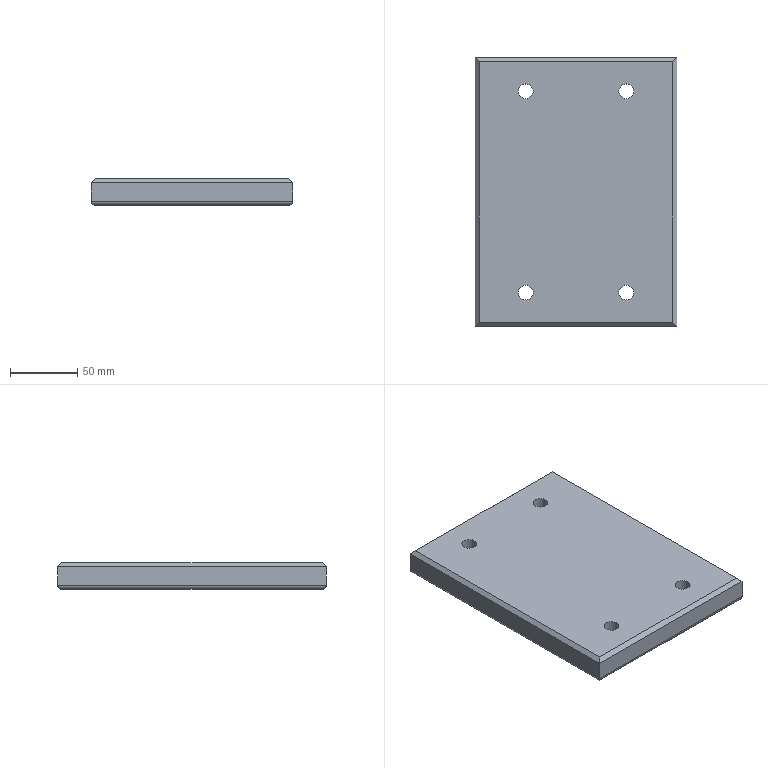Part | NX | features solid 2 | 1 solid | 26 faces | box 150 x 200 x 20 mm | volume 580958 mm3 | plane 14 | cylinder 12 | commonest cylinder face diameters 6 x4 11 x4 17.5 x4
STEP:
#1=CARTESIAN_POINT('',(660.,-340.,317.));
#2=VERTEX_POINT('',#1);
#3=CARTESIAN_POINT('',(660.,-340.,303.));
#4=VERTEX_POINT('',#3);
#5=CARTESIAN_POINT('',(660.,-340.,320.));
#6=DIRECTION('',(0.,0.,-1.));
#7=VECTOR('',#6,1000.);
#8=LINE('',#5,#7);
#9=EDGE_CURVE('',#2,#4,#8,.T.);
#10=ORIENTED_EDGE('',*,*,#9,.T.);
#11=CARTESIAN_POINT('',(510.,-340.,303.));
#12=VERTEX_POINT('',#11);
#13=CARTESIAN_POINT('',(660.,-340.,303.));
#14=DIRECTION('',(1.,0.,0.));
#15=VECTOR('',#14,1000.);
#16=LINE('',#13,#15);
#17=EDGE_CURVE('',#12,#4,#16,.T.);
#18=ORIENTED_EDGE('',*,*,#17,.F.);
#19=CARTESIAN_POINT('',(510.,-340.,317.));
#20=VERTEX_POINT('',#19);
#21=CARTESIAN_POINT('',(510.,-340.,320.));
#22=DIRECTION('',(0.,0.,-1.));
#23=VECTOR('',#22,1000.);
#24=LINE('',#21,#23);
#25=EDGE_CURVE('',#20,#12,#24,.T.);
#26=ORIENTED_EDGE('',*,*,#25,.F.);
#27=CARTESIAN_POINT('',(535.,-340.,317.));
#28=DIRECTION('',(-1.,0.,0.));
#29=VECTOR('',#28,1000.);
#30=LINE('',#27,#29);
#31=EDGE_CURVE('',#2,#20,#30,.T.);
#32=ORIENTED_EDGE('',*,*,#31,.F.);
#33=EDGE_LOOP('',(#10,#18,#26,#32));
#34=FACE_BOUND('',#33,.T.);
#35=CARTESIAN_POINT('',(535.,-340.,320.));
#36=DIRECTION('',(0.,-1.,0.));
#37=DIRECTION('',(-1.,0.,0.));
#38=AXIS2_PLACEMENT_3D('',#35,#36,#37);
#39=PLANE('',#38);
#40=ADVANCED_FACE('',(#34),#39,.F.);
#41=CARTESIAN_POINT('',(660.,-540.,317.));
#42=VERTEX_POINT('',#41);
#43=CARTESIAN_POINT('',(660.,-540.,303.));
#44=VERTEX_POINT('',#43);
#45=CARTESIAN_POINT('',(660.,-540.,320.));
#46=DIRECTION('',(0.,0.,-1.));
#47=VECTOR('',#46,1000.);
#48=LINE('',#45,#47);
#49=EDGE_CURVE('',#42,#44,#48,.T.);
#50=ORIENTED_EDGE('',*,*,#49,.T.);
#51=CARTESIAN_POINT('',(660.,-540.,303.));
#52=DIRECTION('',(0.,-1.,0.));
#53=VECTOR('',#52,1000.);
#54=LINE('',#51,#53);
#55=EDGE_CURVE('',#4,#44,#54,.T.);
#56=ORIENTED_EDGE('',*,*,#55,.F.);
#57=ORIENTED_EDGE('',*,*,#9,.F.);
#58=CARTESIAN_POINT('',(660.,-340.,317.));
#59=DIRECTION('',(0.,1.,0.));
#60=VECTOR('',#59,1000.);
#61=LINE('',#58,#60);
#62=EDGE_CURVE('',#42,#2,#61,.T.);
#63=ORIENTED_EDGE('',*,*,#62,.F.);
#64=EDGE_LOOP('',(#50,#56,#57,#63));
#65=FACE_BOUND('',#64,.T.);
#66=CARTESIAN_POINT('',(660.,-340.,320.));
#67=DIRECTION('',(-1.,0.,0.));
#68=DIRECTION('',(0.,0.,1.));
#69=AXIS2_PLACEMENT_3D('',#66,#67,#68);
#70=PLANE('',#69);
#71=ADVANCED_FACE('',(#65),#70,.F.);
#72=CARTESIAN_POINT('',(510.,-540.,317.));
#73=VERTEX_POINT('',#72);
#74=CARTESIAN_POINT('',(510.,-540.,303.));
#75=VERTEX_POINT('',#74);
#76=CARTESIAN_POINT('',(510.,-540.,320.));
#77=DIRECTION('',(0.,0.,-1.));
#78=VECTOR('',#77,1000.);
#79=LINE('',#76,#78);
#80=EDGE_CURVE('',#73,#75,#79,.T.);
#81=ORIENTED_EDGE('',*,*,#80,.T.);
#82=CARTESIAN_POINT('',(535.,-540.,303.));
#83=DIRECTION('',(-1.,0.,0.));
#84=VECTOR('',#83,1000.);
#85=LINE('',#82,#84);
#86=EDGE_CURVE('',#44,#75,#85,.T.);
#87=ORIENTED_EDGE('',*,*,#86,.F.);
#88=ORIENTED_EDGE('',*,*,#49,.F.);
#89=CARTESIAN_POINT('',(660.,-540.,317.));
#90=DIRECTION('',(1.,0.,0.));
#91=VECTOR('',#90,1000.);
#92=LINE('',#89,#91);
#93=EDGE_CURVE('',#73,#42,#92,.T.);
#94=ORIENTED_EDGE('',*,*,#93,.F.);
#95=EDGE_LOOP('',(#81,#87,#88,#94));
#96=FACE_BOUND('',#95,.T.);
#97=CARTESIAN_POINT('',(660.,-540.,320.));
#98=DIRECTION('',(0.,1.,0.));
#99=DIRECTION('',(0.,0.,1.));
#100=AXIS2_PLACEMENT_3D('',#97,#98,#99);
#101=PLANE('',#100);
#102=ADVANCED_FACE('',(#96),#101,.F.);
#103=ORIENTED_EDGE('',*,*,#25,.T.);
#104=CARTESIAN_POINT('',(510.,-340.,303.));
#105=DIRECTION('',(0.,1.,0.));
#106=VECTOR('',#105,1000.);
#107=LINE('',#104,#106);
#108=EDGE_CURVE('',#75,#12,#107,.T.);
#109=ORIENTED_EDGE('',*,*,#108,.F.);
#110=ORIENTED_EDGE('',*,*,#80,.F.);
#111=CARTESIAN_POINT('',(510.,-540.,317.));
#112=DIRECTION('',(0.,-1.,0.));
#113=VECTOR('',#112,1000.);
#114=LINE('',#111,#113);
#115=EDGE_CURVE('',#20,#73,#114,.T.);
#116=ORIENTED_EDGE('',*,*,#115,.F.);
#117=EDGE_LOOP('',(#103,#109,#110,#116));
#118=FACE_BOUND('',#117,.T.);
#119=CARTESIAN_POINT('',(510.,-540.,320.));
#120=DIRECTION('',(1.,0.,0.));
#121=DIRECTION('',(0.,-1.,0.));
#122=AXIS2_PLACEMENT_3D('',#119,#120,#121);
#123=PLANE('',#122);
#124=ADVANCED_FACE('',(#118),#123,.F.);
#125=CARTESIAN_POINT('',(657.,-343.,320.));
#126=VERTEX_POINT('',#125);
#127=CARTESIAN_POINT('',(657.,-537.,320.));
#128=VERTEX_POINT('',#127);
#129=CARTESIAN_POINT('',(657.,-340.,320.));
#130=DIRECTION('',(0.,-1.,0.));
#131=VECTOR('',#130,1000.);
#132=LINE('',#129,#131);
#133=EDGE_CURVE('',#126,#128,#132,.T.);
#134=ORIENTED_EDGE('',*,*,#133,.F.);
#135=CARTESIAN_POINT('',(513.,-343.,320.));
#136=VERTEX_POINT('',#135);
#137=CARTESIAN_POINT('',(535.,-343.,320.));
#138=DIRECTION('',(1.,0.,0.));
#139=VECTOR('',#138,1000.);
#140=LINE('',#137,#139);
#141=EDGE_CURVE('',#136,#126,#140,.T.);
#142=ORIENTED_EDGE('',*,*,#141,.F.);
#143=CARTESIAN_POINT('',(513.,-537.,320.));
#144=VERTEX_POINT('',#143);
#145=CARTESIAN_POINT('',(513.,-340.,320.));
#146=DIRECTION('',(0.,1.,0.));
#147=VECTOR('',#146,1000.);
#148=LINE('',#145,#147);
#149=EDGE_CURVE('',#144,#136,#148,.T.);
#150=ORIENTED_EDGE('',*,*,#149,.F.);
#151=CARTESIAN_POINT('',(535.,-537.,320.));
#152=DIRECTION('',(-1.,0.,0.));
#153=VECTOR('',#152,1000.);
#154=LINE('',#151,#153);
#155=EDGE_CURVE('',#128,#144,#154,.T.);
#156=ORIENTED_EDGE('',*,*,#155,.F.);
#157=EDGE_LOOP('',(#134,#142,#150,#156));
#158=FACE_BOUND('',#157,.T.);
#159=CARTESIAN_POINT('',(622.5,-509.5,320.));
#160=VERTEX_POINT('',#159);
#161=CARTESIAN_POINT('',(622.5,-515.,320.));
#162=DIRECTION('',(0.,0.,1.));
#163=DIRECTION('',(0.,1.,0.));
#164=AXIS2_PLACEMENT_3D('',#161,#162,#163);
#165=CIRCLE('',#164,5.5);
#166=EDGE_CURVE('',#160,#160,#165,.T.);
#167=ORIENTED_EDGE('',*,*,#166,.F.);
#168=EDGE_LOOP('',(#167));
#169=FACE_BOUND('',#168,.T.);
#170=CARTESIAN_POINT('',(547.5,-509.5,320.));
#171=VERTEX_POINT('',#170);
#172=CARTESIAN_POINT('',(547.5,-515.,320.));
#173=DIRECTION('',(0.,0.,1.));
#174=DIRECTION('',(0.,1.,0.));
#175=AXIS2_PLACEMENT_3D('',#172,#173,#174);
#176=CIRCLE('',#175,5.5);
#177=EDGE_CURVE('',#171,#171,#176,.T.);
#178=ORIENTED_EDGE('',*,*,#177,.F.);
#179=EDGE_LOOP('',(#178));
#180=FACE_BOUND('',#179,.T.);
#181=CARTESIAN_POINT('',(622.5,-359.5,320.));
#182=VERTEX_POINT('',#181);
#183=CARTESIAN_POINT('',(622.5,-365.,320.));
#184=DIRECTION('',(0.,0.,1.));
#185=DIRECTION('',(0.,1.,0.));
#186=AXIS2_PLACEMENT_3D('',#183,#184,#185);
#187=CIRCLE('',#186,5.5);
#188=EDGE_CURVE('',#182,#182,#187,.T.);
#189=ORIENTED_EDGE('',*,*,#188,.F.);
#190=EDGE_LOOP('',(#189));
#191=FACE_BOUND('',#190,.T.);
#192=CARTESIAN_POINT('',(547.5,-359.5,320.));
#193=VERTEX_POINT('',#192);
#194=CARTESIAN_POINT('',(547.5,-365.,320.));
#195=DIRECTION('',(0.,0.,1.));
#196=DIRECTION('',(0.,1.,0.));
#197=AXIS2_PLACEMENT_3D('',#194,#195,#196);
#198=CIRCLE('',#197,5.5);
#199=EDGE_CURVE('',#193,#193,#198,.T.);
#200=ORIENTED_EDGE('',*,*,#199,.F.);
#201=EDGE_LOOP('',(#200));
#202=FACE_BOUND('',#201,.T.);
#203=CARTESIAN_POINT('',(535.,-340.,320.));
#204=DIRECTION('',(0.,0.,-1.));
#205=DIRECTION('',(0.,1.,0.));
#206=AXIS2_PLACEMENT_3D('',#203,#204,#205);
#207=PLANE('',#206);
#208=ADVANCED_FACE('',(#158,#169,#180,#191,#202),#207,.F.);
#209=CARTESIAN_POINT('',(657.,-343.,300.));
#210=VERTEX_POINT('',#209);
#211=CARTESIAN_POINT('',(513.,-343.,300.));
#212=VERTEX_POINT('',#211);
#213=CARTESIAN_POINT('',(535.,-343.,300.));
#214=DIRECTION('',(1.,0.,0.));
#215=VECTOR('',#214,1000.);
#216=LINE('',#213,#215);
#217=EDGE_CURVE('',#210,#212,#216,.F.);
#218=ORIENTED_EDGE('',*,*,#217,.F.);
#219=CARTESIAN_POINT('',(657.,-537.,300.));
#220=VERTEX_POINT('',#219);
#221=CARTESIAN_POINT('',(657.,-340.,300.));
#222=DIRECTION('',(0.,-1.,0.));
#223=VECTOR('',#222,1000.);
#224=LINE('',#221,#223);
#225=EDGE_CURVE('',#220,#210,#224,.F.);
#226=ORIENTED_EDGE('',*,*,#225,.F.);
#227=CARTESIAN_POINT('',(513.,-537.,300.));
#228=VERTEX_POINT('',#227);
#229=CARTESIAN_POINT('',(660.,-537.,300.));
#230=DIRECTION('',(-1.,0.,0.));
#231=VECTOR('',#230,1000.);
#232=LINE('',#229,#231);
#233=EDGE_CURVE('',#228,#220,#232,.F.);
#234=ORIENTED_EDGE('',*,*,#233,.F.);
#235=CARTESIAN_POINT('',(513.,-540.,300.));
#236=DIRECTION('',(0.,1.,0.));
#237=VECTOR('',#236,1000.);
#238=LINE('',#235,#237);
#239=EDGE_CURVE('',#212,#228,#238,.F.);
#240=ORIENTED_EDGE('',*,*,#239,.F.);
#241=EDGE_LOOP('',(#218,#226,#234,#240));
#242=FACE_BOUND('',#241,.T.);
#243=CARTESIAN_POINT('',(622.5,-523.75,300.));
#244=VERTEX_POINT('',#243);
#245=CARTESIAN_POINT('',(622.5,-515.,300.));
#246=DIRECTION('',(0.,0.,-1.));
#247=DIRECTION('',(0.,-1.,0.));
#248=AXIS2_PLACEMENT_3D('',#245,#246,#247);
#249=CIRCLE('',#248,8.75);
#250=EDGE_CURVE('',#244,#244,#249,.T.);
#251=ORIENTED_EDGE('',*,*,#250,.F.);
#252=EDGE_LOOP('',(#251));
#253=FACE_BOUND('',#252,.T.);
#254=CARTESIAN_POINT('',(547.5,-523.75,300.));
#255=VERTEX_POINT('',#254);
#256=CARTESIAN_POINT('',(547.5,-515.,300.));
#257=DIRECTION('',(0.,0.,-1.));
#258=DIRECTION('',(0.,-1.,0.));
#259=AXIS2_PLACEMENT_3D('',#256,#257,#258);
#260=CIRCLE('',#259,8.75);
#261=EDGE_CURVE('',#255,#255,#260,.T.);
#262=ORIENTED_EDGE('',*,*,#261,.F.);
#263=EDGE_LOOP('',(#262));
#264=FACE_BOUND('',#263,.T.);
#265=CARTESIAN_POINT('',(622.5,-373.75,300.));
#266=VERTEX_POINT('',#265);
#267=CARTESIAN_POINT('',(622.5,-365.,300.));
#268=DIRECTION('',(0.,0.,-1.));
#269=DIRECTION('',(0.,-1.,0.));
#270=AXIS2_PLACEMENT_3D('',#267,#268,#269);
#271=CIRCLE('',#270,8.75);
#272=EDGE_CURVE('',#266,#266,#271,.T.);
#273=ORIENTED_EDGE('',*,*,#272,.F.);
#274=EDGE_LOOP('',(#273));
#275=FACE_BOUND('',#274,.T.);
#276=CARTESIAN_POINT('',(547.5,-373.75,300.));
#277=VERTEX_POINT('',#276);
#278=CARTESIAN_POINT('',(547.5,-365.,300.));
#279=DIRECTION('',(0.,0.,-1.));
#280=DIRECTION('',(0.,-1.,0.));
#281=AXIS2_PLACEMENT_3D('',#278,#279,#280);
#282=CIRCLE('',#281,8.75);
#283=EDGE_CURVE('',#277,#277,#282,.T.);
#284=ORIENTED_EDGE('',*,*,#283,.F.);
#285=EDGE_LOOP('',(#284));
#286=FACE_BOUND('',#285,.T.);
#287=CARTESIAN_POINT('',(535.,-340.,300.));
#288=DIRECTION('',(0.,0.,-1.));
#289=DIRECTION('',(0.,1.,0.));
#290=AXIS2_PLACEMENT_3D('',#287,#288,#289);
#291=PLANE('',#290);
#292=ADVANCED_FACE('',(#242,#253,#264,#275,#286),#291,.T.);
#293=CARTESIAN_POINT('',(547.5,-370.5,312.));
#294=VERTEX_POINT('',#293);
#295=CARTESIAN_POINT('',(547.5,-365.,312.));
#296=DIRECTION('',(0.,0.,-1.));
#297=DIRECTION('',(0.,-1.,0.));
#298=AXIS2_PLACEMENT_3D('',#295,#296,#297);
#299=CIRCLE('',#298,5.5);
#300=EDGE_CURVE('',#294,#294,#299,.T.);
#301=ORIENTED_EDGE('',*,*,#300,.T.);
#302=EDGE_LOOP('',(#301));
#303=FACE_BOUND('',#302,.T.);
#304=ORIENTED_EDGE('',*,*,#199,.T.);
#305=EDGE_LOOP('',(#304));
#306=FACE_BOUND('',#305,.T.);
#307=CARTESIAN_POINT('',(547.5,-365.,350.));
#308=DIRECTION('',(0.,0.,1.));
#309=DIRECTION('',(0.,-1.,0.));
#310=AXIS2_PLACEMENT_3D('',#307,#308,#309);
#311=CYLINDRICAL_SURFACE('',#310,5.5);
#312=ADVANCED_FACE('',(#303,#306),#311,.F.);
#313=ORIENTED_EDGE('',*,*,#300,.F.);
#314=EDGE_LOOP('',(#313));
#315=FACE_BOUND('',#314,.T.);
#316=CARTESIAN_POINT('',(547.5,-373.75,312.));
#317=VERTEX_POINT('',#316);
#318=CARTESIAN_POINT('',(547.5,-365.,312.));
#319=DIRECTION('',(0.,0.,-1.));
#320=DIRECTION('',(0.,-1.,0.));
#321=AXIS2_PLACEMENT_3D('',#318,#319,#320);
#322=CIRCLE('',#321,8.75);
#323=EDGE_CURVE('',#317,#317,#322,.T.);
#324=ORIENTED_EDGE('',*,*,#323,.T.);
#325=EDGE_LOOP('',(#324));
#326=FACE_BOUND('',#325,.T.);
#327=CARTESIAN_POINT('',(547.5,-365.,312.));
#328=DIRECTION('',(0.,0.,1.));
#329=DIRECTION('',(0.,-1.,0.));
#330=AXIS2_PLACEMENT_3D('',#327,#328,#329);
#331=PLANE('',#330);
#332=ADVANCED_FACE('',(#315,#326),#331,.F.);
#333=ORIENTED_EDGE('',*,*,#323,.F.);
#334=EDGE_LOOP('',(#333));
#335=FACE_BOUND('',#334,.T.);
#336=ORIENTED_EDGE('',*,*,#283,.T.);
#337=EDGE_LOOP('',(#336));
#338=FACE_BOUND('',#337,.T.);
#339=CARTESIAN_POINT('',(547.5,-365.,300.));
#340=DIRECTION('',(0.,0.,1.));
#341=DIRECTION('',(0.,-1.,0.));
#342=AXIS2_PLACEMENT_3D('',#339,#340,#341);
#343=CYLINDRICAL_SURFACE('',#342,8.75);
#344=ADVANCED_FACE('',(#335,#338),#343,.F.);
#345=CARTESIAN_POINT('',(622.5,-370.5,312.));
#346=VERTEX_POINT('',#345);
#347=CARTESIAN_POINT('',(622.5,-365.,312.));
#348=DIRECTION('',(0.,0.,-1.));
#349=DIRECTION('',(0.,-1.,0.));
#350=AXIS2_PLACEMENT_3D('',#347,#348,#349);
#351=CIRCLE('',#350,5.5);
#352=EDGE_CURVE('',#346,#346,#351,.T.);
#353=ORIENTED_EDGE('',*,*,#352,.T.);
#354=EDGE_LOOP('',(#353));
#355=FACE_BOUND('',#354,.T.);
#356=ORIENTED_EDGE('',*,*,#188,.T.);
#357=EDGE_LOOP('',(#356));
#358=FACE_BOUND('',#357,.T.);
#359=CARTESIAN_POINT('',(622.5,-365.,350.));
#360=DIRECTION('',(0.,0.,1.));
#361=DIRECTION('',(0.,-1.,0.));
#362=AXIS2_PLACEMENT_3D('',#359,#360,#361);
#363=CYLINDRICAL_SURFACE('',#362,5.5);
#364=ADVANCED_FACE('',(#355,#358),#363,.F.);
#365=ORIENTED_EDGE('',*,*,#352,.F.);
#366=EDGE_LOOP('',(#365));
#367=FACE_BOUND('',#366,.T.);
#368=CARTESIAN_POINT('',(622.5,-373.75,312.));
#369=VERTEX_POINT('',#368);
#370=CARTESIAN_POINT('',(622.5,-365.,312.));
#371=DIRECTION('',(0.,0.,-1.));
#372=DIRECTION('',(0.,-1.,0.));
#373=AXIS2_PLACEMENT_3D('',#370,#371,#372);
#374=CIRCLE('',#373,8.75);
#375=EDGE_CURVE('',#369,#369,#374,.T.);
#376=ORIENTED_EDGE('',*,*,#375,.T.);
#377=EDGE_LOOP('',(#376));
#378=FACE_BOUND('',#377,.T.);
#379=CARTESIAN_POINT('',(622.5,-365.,312.));
#380=DIRECTION('',(0.,0.,1.));
#381=DIRECTION('',(0.,-1.,0.));
#382=AXIS2_PLACEMENT_3D('',#379,#380,#381);
#383=PLANE('',#382);
#384=ADVANCED_FACE('',(#367,#378),#383,.F.);
#385=ORIENTED_EDGE('',*,*,#375,.F.);
#386=EDGE_LOOP('',(#385));
#387=FACE_BOUND('',#386,.T.);
#388=ORIENTED_EDGE('',*,*,#272,.T.);
#389=EDGE_LOOP('',(#388));
#390=FACE_BOUND('',#389,.T.);
#391=CARTESIAN_POINT('',(622.5,-365.,300.));
#392=DIRECTION('',(0.,0.,1.));
#393=DIRECTION('',(0.,-1.,0.));
#394=AXIS2_PLACEMENT_3D('',#391,#392,#393);
#395=CYLINDRICAL_SURFACE('',#394,8.75);
#396=ADVANCED_FACE('',(#387,#390),#395,.F.);
#397=CARTESIAN_POINT('',(547.5,-520.5,312.));
#398=VERTEX_POINT('',#397);
#399=CARTESIAN_POINT('',(547.5,-515.,312.));
#400=DIRECTION('',(0.,0.,-1.));
#401=DIRECTION('',(0.,-1.,0.));
#402=AXIS2_PLACEMENT_3D('',#399,#400,#401);
#403=CIRCLE('',#402,5.5);
#404=EDGE_CURVE('',#398,#398,#403,.T.);
#405=ORIENTED_EDGE('',*,*,#404,.T.);
#406=EDGE_LOOP('',(#405));
#407=FACE_BOUND('',#406,.T.);
#408=ORIENTED_EDGE('',*,*,#177,.T.);
#409=EDGE_LOOP('',(#408));
#410=FACE_BOUND('',#409,.T.);
#411=CARTESIAN_POINT('',(547.5,-515.,350.));
#412=DIRECTION('',(0.,0.,1.));
#413=DIRECTION('',(0.,-1.,0.));
#414=AXIS2_PLACEMENT_3D('',#411,#412,#413);
#415=CYLINDRICAL_SURFACE('',#414,5.5);
#416=ADVANCED_FACE('',(#407,#410),#415,.F.);
#417=ORIENTED_EDGE('',*,*,#404,.F.);
#418=EDGE_LOOP('',(#417));
#419=FACE_BOUND('',#418,.T.);
#420=CARTESIAN_POINT('',(547.5,-523.75,312.));
#421=VERTEX_POINT('',#420);
#422=CARTESIAN_POINT('',(547.5,-515.,312.));
#423=DIRECTION('',(0.,0.,-1.));
#424=DIRECTION('',(0.,-1.,0.));
#425=AXIS2_PLACEMENT_3D('',#422,#423,#424);
#426=CIRCLE('',#425,8.75);
#427=EDGE_CURVE('',#421,#421,#426,.T.);
#428=ORIENTED_EDGE('',*,*,#427,.T.);
#429=EDGE_LOOP('',(#428));
#430=FACE_BOUND('',#429,.T.);
#431=CARTESIAN_POINT('',(547.5,-515.,312.));
#432=DIRECTION('',(0.,0.,1.));
#433=DIRECTION('',(0.,-1.,0.));
#434=AXIS2_PLACEMENT_3D('',#431,#432,#433);
#435=PLANE('',#434);
#436=ADVANCED_FACE('',(#419,#430),#435,.F.);
#437=ORIENTED_EDGE('',*,*,#427,.F.);
#438=EDGE_LOOP('',(#437));
#439=FACE_BOUND('',#438,.T.);
#440=ORIENTED_EDGE('',*,*,#261,.T.);
#441=EDGE_LOOP('',(#440));
#442=FACE_BOUND('',#441,.T.);
#443=CARTESIAN_POINT('',(547.5,-515.,300.));
#444=DIRECTION('',(0.,0.,1.));
#445=DIRECTION('',(0.,-1.,0.));
#446=AXIS2_PLACEMENT_3D('',#443,#444,#445);
#447=CYLINDRICAL_SURFACE('',#446,8.75);
#448=ADVANCED_FACE('',(#439,#442),#447,.F.);
#449=CARTESIAN_POINT('',(622.5,-520.5,312.));
#450=VERTEX_POINT('',#449);
#451=CARTESIAN_POINT('',(622.5,-515.,312.));
#452=DIRECTION('',(0.,0.,-1.));
#453=DIRECTION('',(0.,-1.,0.));
#454=AXIS2_PLACEMENT_3D('',#451,#452,#453);
#455=CIRCLE('',#454,5.5);
#456=EDGE_CURVE('',#450,#450,#455,.T.);
#457=ORIENTED_EDGE('',*,*,#456,.T.);
#458=EDGE_LOOP('',(#457));
#459=FACE_BOUND('',#458,.T.);
#460=ORIENTED_EDGE('',*,*,#166,.T.);
#461=EDGE_LOOP('',(#460));
#462=FACE_BOUND('',#461,.T.);
#463=CARTESIAN_POINT('',(622.5,-515.,350.));
#464=DIRECTION('',(0.,0.,1.));
#465=DIRECTION('',(0.,-1.,0.));
#466=AXIS2_PLACEMENT_3D('',#463,#464,#465);
#467=CYLINDRICAL_SURFACE('',#466,5.5);
#468=ADVANCED_FACE('',(#459,#462),#467,.F.);
#469=ORIENTED_EDGE('',*,*,#456,.F.);
#470=EDGE_LOOP('',(#469));
#471=FACE_BOUND('',#470,.T.);
#472=CARTESIAN_POINT('',(622.5,-523.75,312.));
#473=VERTEX_POINT('',#472);
#474=CARTESIAN_POINT('',(622.5,-515.,312.));
#475=DIRECTION('',(0.,0.,-1.));
#476=DIRECTION('',(0.,-1.,0.));
#477=AXIS2_PLACEMENT_3D('',#474,#475,#476);
#478=CIRCLE('',#477,8.75);
#479=EDGE_CURVE('',#473,#473,#478,.T.);
#480=ORIENTED_EDGE('',*,*,#479,.T.);
#481=EDGE_LOOP('',(#480));
#482=FACE_BOUND('',#481,.T.);
#483=CARTESIAN_POINT('',(622.5,-515.,312.));
#484=DIRECTION('',(0.,0.,1.));
#485=DIRECTION('',(0.,-1.,0.));
#486=AXIS2_PLACEMENT_3D('',#483,#484,#485);
#487=PLANE('',#486);
#488=ADVANCED_FACE('',(#471,#482),#487,.F.);
#489=ORIENTED_EDGE('',*,*,#479,.F.);
#490=EDGE_LOOP('',(#489));
#491=FACE_BOUND('',#490,.T.);
#492=ORIENTED_EDGE('',*,*,#250,.T.);
#493=EDGE_LOOP('',(#492));
#494=FACE_BOUND('',#493,.T.);
#495=CARTESIAN_POINT('',(622.5,-515.,300.));
#496=DIRECTION('',(0.,0.,1.));
#497=DIRECTION('',(0.,-1.,0.));
#498=AXIS2_PLACEMENT_3D('',#495,#496,#497);
#499=CYLINDRICAL_SURFACE('',#498,8.75);
#500=ADVANCED_FACE('',(#491,#494),#499,.F.);
#501=CARTESIAN_POINT('',(657.,-343.,303.));
#502=DIRECTION('',(0.7071,-0.7071,0.));
#503=DIRECTION('',(-0.7071,-0.7071,0.));
#504=AXIS2_PLACEMENT_3D('',#501,#502,#503);
#505=ELLIPSE('',#504,4.243,3.);
#506=EDGE_CURVE('',#210,#4,#505,.T.);
#507=ORIENTED_EDGE('',*,*,#506,.T.);
#508=ORIENTED_EDGE('',*,*,#55,.T.);
#509=CARTESIAN_POINT('',(657.,-537.,303.));
#510=DIRECTION('',(-0.7071,-0.7071,0.));
#511=DIRECTION('',(-0.7071,0.7071,0.));
#512=AXIS2_PLACEMENT_3D('',#509,#510,#511);
#513=ELLIPSE('',#512,4.243,3.);
#514=EDGE_CURVE('',#44,#220,#513,.F.);
#515=ORIENTED_EDGE('',*,*,#514,.T.);
#516=ORIENTED_EDGE('',*,*,#225,.T.);
#517=EDGE_LOOP('',(#507,#508,#515,#516));
#518=FACE_BOUND('',#517,.T.);
#519=CARTESIAN_POINT('',(657.,-340.,303.));
#520=DIRECTION('',(0.,1.,0.));
#521=DIRECTION('',(0.,0.,1.));
#522=AXIS2_PLACEMENT_3D('',#519,#520,#521);
#523=CYLINDRICAL_SURFACE('',#522,3.);
#524=ADVANCED_FACE('',(#518),#523,.T.);
#525=ORIENTED_EDGE('',*,*,#514,.F.);
#526=ORIENTED_EDGE('',*,*,#86,.T.);
#527=CARTESIAN_POINT('',(513.,-537.,303.));
#528=DIRECTION('',(-0.7071,0.7071,0.));
#529=DIRECTION('',(0.7071,0.7071,0.));
#530=AXIS2_PLACEMENT_3D('',#527,#528,#529);
#531=ELLIPSE('',#530,4.243,3.);
#532=EDGE_CURVE('',#75,#228,#531,.F.);
#533=ORIENTED_EDGE('',*,*,#532,.T.);
#534=ORIENTED_EDGE('',*,*,#233,.T.);
#535=EDGE_LOOP('',(#525,#526,#533,#534));
#536=FACE_BOUND('',#535,.T.);
#537=CARTESIAN_POINT('',(660.,-537.,303.));
#538=DIRECTION('',(1.,0.,0.));
#539=DIRECTION('',(0.,0.,-1.));
#540=AXIS2_PLACEMENT_3D('',#537,#538,#539);
#541=CYLINDRICAL_SURFACE('',#540,3.);
#542=ADVANCED_FACE('',(#536),#541,.T.);
#543=ORIENTED_EDGE('',*,*,#506,.F.);
#544=ORIENTED_EDGE('',*,*,#217,.T.);
#545=CARTESIAN_POINT('',(513.,-343.,303.));
#546=DIRECTION('',(0.7071,0.7071,0.));
#547=DIRECTION('',(-0.7071,0.7071,0.));
#548=AXIS2_PLACEMENT_3D('',#545,#546,#547);
#549=ELLIPSE('',#548,4.243,3.);
#550=EDGE_CURVE('',#212,#12,#549,.T.);
#551=ORIENTED_EDGE('',*,*,#550,.T.);
#552=ORIENTED_EDGE('',*,*,#17,.T.);
#553=EDGE_LOOP('',(#543,#544,#551,#552));
#554=FACE_BOUND('',#553,.T.);
#555=CARTESIAN_POINT('',(535.,-343.,303.));
#556=DIRECTION('',(-1.,0.,0.));
#557=DIRECTION('',(0.,1.,0.));
#558=AXIS2_PLACEMENT_3D('',#555,#556,#557);
#559=CYLINDRICAL_SURFACE('',#558,3.);
#560=ADVANCED_FACE('',(#554),#559,.T.);
#561=ORIENTED_EDGE('',*,*,#532,.F.);
#562=ORIENTED_EDGE('',*,*,#108,.T.);
#563=ORIENTED_EDGE('',*,*,#550,.F.);
#564=ORIENTED_EDGE('',*,*,#239,.T.);
#565=EDGE_LOOP('',(#561,#562,#563,#564));
#566=FACE_BOUND('',#565,.T.);
#567=CARTESIAN_POINT('',(513.,-540.,303.));
#568=DIRECTION('',(0.,-1.,0.));
#569=DIRECTION('',(-1.,0.,0.));
#570=AXIS2_PLACEMENT_3D('',#567,#568,#569);
#571=CYLINDRICAL_SURFACE('',#570,3.);
#572=ADVANCED_FACE('',(#566),#571,.T.);
#573=CARTESIAN_POINT('',(512.,-342.,319.));
#574=DIRECTION('',(0.5774,-0.5774,0.5774));
#575=VECTOR('',#574,1000.);
#576=LINE('',#573,#575);
#577=EDGE_CURVE('',#20,#136,#576,.T.);
#578=ORIENTED_EDGE('',*,*,#577,.T.);
#579=ORIENTED_EDGE('',*,*,#141,.T.);
#580=CARTESIAN_POINT('',(616.333,-383.667,360.667));
#581=DIRECTION('',(-0.5774,-0.5774,0.5774));
#582=VECTOR('',#581,1000.);
#583=LINE('',#580,#582);
#584=EDGE_CURVE('',#126,#2,#583,.F.);
#585=ORIENTED_EDGE('',*,*,#584,.T.);
#586=ORIENTED_EDGE('',*,*,#31,.T.);
#587=EDGE_LOOP('',(#578,#579,#585,#586));
#588=FACE_BOUND('',#587,.T.);
#589=CARTESIAN_POINT('',(535.,-343.,320.));
#590=DIRECTION('',(0.,-0.7071,-0.7071));
#591=DIRECTION('',(0.,0.7071,-0.7071));
#592=AXIS2_PLACEMENT_3D('',#589,#590,#591);
#593=PLANE('',#592);
#594=ADVANCED_FACE('',(#588),#593,.F.);
#595=ORIENTED_EDGE('',*,*,#584,.F.);
#596=ORIENTED_EDGE('',*,*,#133,.T.);
#597=CARTESIAN_POINT('',(591.333,-471.333,385.667));
#598=DIRECTION('',(-0.5774,0.5774,0.5774));
#599=VECTOR('',#598,1000.);
#600=LINE('',#597,#599);
#601=EDGE_CURVE('',#128,#42,#600,.F.);
#602=ORIENTED_EDGE('',*,*,#601,.T.);
#603=ORIENTED_EDGE('',*,*,#62,.T.);
#604=EDGE_LOOP('',(#595,#596,#602,#603));
#605=FACE_BOUND('',#604,.T.);
#606=CARTESIAN_POINT('',(657.,-340.,320.));
#607=DIRECTION('',(-0.7071,0.,-0.7071));
#608=DIRECTION('',(-0.7071,0.,0.7071));
#609=AXIS2_PLACEMENT_3D('',#606,#607,#608);
#610=PLANE('',#609);
#611=ADVANCED_FACE('',(#605),#610,.F.);
#612=ORIENTED_EDGE('',*,*,#577,.F.);
#613=ORIENTED_EDGE('',*,*,#115,.T.);
#614=CARTESIAN_POINT('',(578.667,-471.333,385.667));
#615=DIRECTION('',(-0.5774,-0.5774,-0.5774));
#616=VECTOR('',#615,1000.);
#617=LINE('',#614,#616);
#618=EDGE_CURVE('',#73,#144,#617,.F.);
#619=ORIENTED_EDGE('',*,*,#618,.T.);
#620=ORIENTED_EDGE('',*,*,#149,.T.);
#621=EDGE_LOOP('',(#612,#613,#619,#620));
#622=FACE_BOUND('',#621,.T.);
#623=CARTESIAN_POINT('',(513.,-340.,320.));
#624=DIRECTION('',(0.7071,0.,-0.7071));
#625=DIRECTION('',(-0.7071,0.,-0.7071));
#626=AXIS2_PLACEMENT_3D('',#623,#624,#625);
#627=PLANE('',#626);
#628=ADVANCED_FACE('',(#622),#627,.F.);
#629=ORIENTED_EDGE('',*,*,#601,.F.);
#630=ORIENTED_EDGE('',*,*,#155,.T.);
#631=ORIENTED_EDGE('',*,*,#618,.F.);
#632=ORIENTED_EDGE('',*,*,#93,.T.);
#633=EDGE_LOOP('',(#629,#630,#631,#632));
#634=FACE_BOUND('',#633,.T.);
#635=CARTESIAN_POINT('',(535.,-537.,320.));
#636=DIRECTION('',(0.,0.7071,-0.7071));
#637=DIRECTION('',(0.,0.7071,0.7071));
#638=AXIS2_PLACEMENT_3D('',#635,#636,#637);
#639=PLANE('',#638);
#640=ADVANCED_FACE('',(#634),#639,.F.);
#641=CLOSED_SHELL('',(#40,#71,#102,#124,#208,#292,#312,#332,#344,#364,#384,#396,#416,#436,#448,#468,#488,#500,#524,#542,#560,#572,#594,#611,#628,#640));
#642=MANIFOLD_SOLID_BREP('',#641);
#643=(LENGTH_UNIT()NAMED_UNIT(*)SI_UNIT(.MILLI.,.METRE.));
#644=UNCERTAINTY_MEASURE_WITH_UNIT(LENGTH_MEASURE(0.00001),#643,'','');
#645=(NAMED_UNIT(*)PLANE_ANGLE_UNIT()SI_UNIT($,.RADIAN.));
#646=(NAMED_UNIT(*)SI_UNIT($,.STERADIAN.)SOLID_ANGLE_UNIT());
#647=(GEOMETRIC_REPRESENTATION_CONTEXT(3)GLOBAL_UNCERTAINTY_ASSIGNED_CONTEXT((#644))GLOBAL_UNIT_ASSIGNED_CONTEXT((#643,#645,#646))REPRESENTATION_CONTEXT('',''));
#648=ADVANCED_BREP_SHAPE_REPRESENTATION('',(#642),#647);